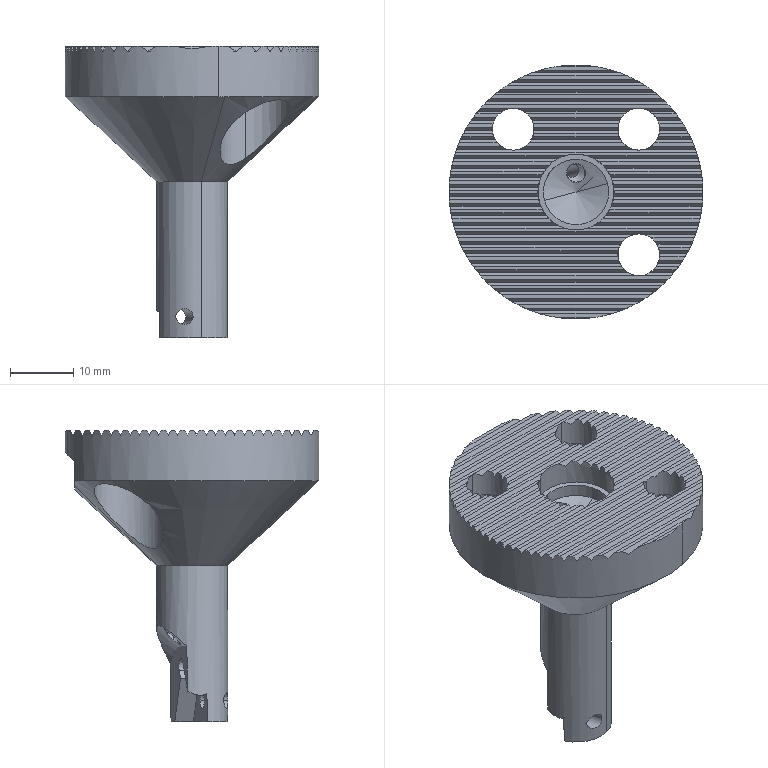Part | 1 solid | 187 faces | box 40 x 40 x 46 mm | volume 15458 mm3 | plane 154 | cylinder 27 | cone 6 | commonest cylinder face diameters 6.6 x6 11 x6 2 x2 2.5 x2 3 x2 10.3 x2